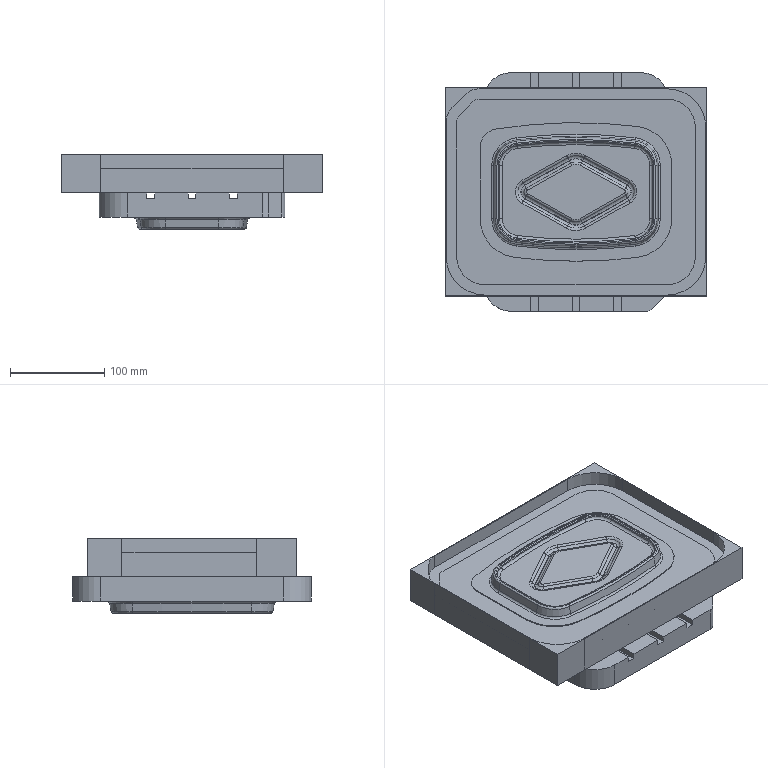NC program | NX | posted with a generic post | part box 278.144 x 254.144 x 79 mm
Lines 4921 to 5862 of 124328:
(CONTOUR_AREA_1 , TOOL : R2)
N9834 M6
N9836 G53
N9838 G17 G0 G90 X-4.674 Y-0.007 S8000 M3 M8
N9840 G43 Z100.5 H0
N9842 Z36.98
N9844 G94 G1 Z33.98 F4500.
N9846 G3 X4.675 Y0.005 R63.773
N9848 G1 X4.673 Y0.006
N9850 G3 X-0.193 Y0.163 R72.733
N9852 X-4.674 Y-0.007 R101.082
N9854 G1 X-8.51 Y-0.148
N9856 X-7.093 Y-0.193
N9858 X-6.747 Y-0.204
N9860 X-5.711 Y-0.244
N9862 G3 X2.733 Y-0.382 R74.506
N9864 G1 X6.059 Y-0.224
N9866 X8.48 Y-0.141
N9868 X11.596 Y-0.07
N9870 X13.848 Y0.003
N9872 X13.852 Y0.004
N9874 X11.743 Y0.077
N9876 G2 X1.804 Y0.42 R263.458
N9878 G3 X-3.288 Y0.349 R55.344
N9880 G1 X-5.646 Y0.238
N9882 X-8.203 Y0.16
N9884 X-13.845 Y0.001
N9886 X-11.249 Y-0.085
N9888 X-8.51 Y-0.148
N9890 X-8.519 Y-0.432
N9892 X-7.056 Y-0.479
N9894 X-6.721 Y-0.49
N9896 X-5.71 Y-0.529
N9898 G3 X2.942 Y-0.657 R74.079
N9900 G1 X5.712 Y-0.522
N9902 X8.576 Y-0.423
N9904 X11.596 Y-0.355
N9906 X20.353 Y-0.069
N9908 X21.805 Y-0.001
N9910 X21.812 Y0.003
N9912 X21.811 Y0.004
N9914 X21.662 Y0.019
N9916 X21.633 Y0.021
N9918 X20.164 Y0.088
N9920 X11.446 Y0.37
N9922 X9.073 Y0.419
N9924 X8.48 Y0.433
N9926 X6.051 Y0.513
N9928 X2.745 Y0.668
N9930 G3 X-2.942 Y0.651 R53.586
N9932 G1 X-5.712 Y0.521
N9934 X-6.784 Y0.485
N9936 X-8.03 Y0.45
N9938 X-16.097 Y0.225
N9940 X-19.624 Y0.105
N9942 X-21.806 Y0.002
N9944 X-20.941 Y-0.044
N9946 X-20.387 Y-0.068
N9948 X-20.153 Y-0.078
N9950 X-11.104 Y-0.373
N9952 X-8.519 Y-0.432
N9954 X-8.528 Y-0.717
N9956 X-7.096 Y-0.763
N9958 X-6.662 Y-0.778
N9960 X-5.711 Y-0.815
N9962 G3 X2.861 Y-0.947 R74.273
N9964 G1 X5.771 Y-0.805
N9966 X8.639 Y-0.707
N9968 X11.596 Y-0.641
N9970 X20.417 Y-0.351
N9972 X22.672 Y-0.244
N9974 X27.347 Y0.002
N9976 X21.101 Y0.333
N9978 X20.105 Y0.375
N9980 X11.387 Y0.656
N9982 X8.134 Y0.728
N9984 X5.993 Y0.801
N9986 X2.596 Y0.96
N9988 X1.015 Y1.014
N9990 X0.331 Y1.023
N9992 X-1.211 Y0.998
N9994 X-2.596 Y0.951
N9996 X-5.773 Y0.804
N9998 X-6.75 Y0.771
N10000 X-8.826 Y0.713
N10002 X-16.104 Y0.51
N10004 X-19.557 Y0.393
N10006 X-22.672 Y0.249
N10008 X-27.341 Y0.006
N10010 X-27.172 Y-0.01
N10012 G3 X-8.528 Y-0.717 R468.382
N10014 G1 X-8.537 Y-1.002
N10016 X-6.057 Y-1.086
N10018 G3 X1.558 Y-1.282 R81.793
N10020 G1 X2.599 Y-1.245
N10022 X5.834 Y-1.088
N10024 X8.345 Y-1.
N10026 G3 X29.624 Y-0.144 R470.604
N10028 G1 X29.619 Y0.027
N10030 X29.594 Y0.147
N10032 X29.578 Y0.157
N10034 X29.416 Y0.173
N10036 X28.21 Y0.244
N10038 G3 X8.134 Y1.014 R451.313
N10040 G1 X5.935 Y1.089
N10042 X4.613 Y1.152
N10044 G3 X-1.905 Y1.263 R62.851
N10046 G1 X-2.253 Y1.251
N10048 X-2.944 Y1.222
N10050 X-5.835 Y1.087
N10052 X-8.826 Y0.997
N10054 G3 X-29.609 Y0.158 R503.183
N10056 G1 X-29.661 Y0.108
N10058 X-29.674 Y0.094
N10060 X-29.655 Y-0.033
N10062 X-29.594 Y-0.142
N10064 X-29.574 Y-0.153
N10066 X-29.364 Y-0.173
N10068 G3 X-8.537 Y-1.002 R491.866
N10070 G1 X-8.546 Y-1.287
N10072 X-6.057 Y-1.372
N10074 G3 X1.214 Y-1.579 R86.109
N10076 G1 X2.624 Y-1.529
N10078 X5.897 Y-1.371
N10080 X8.408 Y-1.283
N10082 G3 X29.683 Y-0.431 R486.038
N10084 G1 X29.842 Y-0.398
N10086 X29.899 Y-0.214
N10088 X29.961 Y0.193
N10090 X29.941 Y0.398
N10092 X29.839 Y0.418
N10094 X29.594 Y0.446
N10096 G3 X8.48 Y1.288 R447.781
N10098 G1 X6.209 Y1.363
N10100 G3 X0.516 Y1.594 R157.649
N10102 X-5.899 Y1.37 R117.358
N10104 G1 X-10.214 Y1.243
N10106 G3 X-29.681 Y0.433 R462.283
N10108 G1 X-29.941 Y0.36
N10110 X-29.973 Y0.141
N10112 X-29.964 Y-0.173
N10114 X-29.963 Y-0.196
N10116 X-29.941 Y-0.335
N10118 X-29.829 Y-0.407
N10120 X-29.594 Y-0.439
N10122 X-29.523 Y-0.447
N10124 G3 X-8.546 Y-1.287 R488.305
N10126 G1 X-8.555 Y-1.571
N10128 X-6.057 Y-1.657
N10130 G3 X1.252 Y-1.863 R85.774
N10132 G1 X2.689 Y-1.811
N10134 X6.057 Y-1.65
N10136 X8.482 Y-1.566
N10138 G3 X30.117 Y-0.689 R483.031
N10140 G1 X30.238 Y0.124
N10142 X30.242 Y0.173
N10144 X30.256 Y0.488
N10146 X30.251 Y0.519
N10148 X30.215 Y0.645
N10150 X30.1 Y0.678
N10152 X29.941 Y0.705
N10154 X29.796 Y0.72
N10156 G3 X19.554 Y1.249 R696.433
N10158 G1 X11.547 Y1.508
N10160 G2 X1.845 Y1.844 R245.456
N10162 G3 X-3.059 Y1.787 R52.345
N10164 G1 X-5.365 Y1.678
N10166 X-5.602 Y1.667
N10168 X-6.057 Y1.65
N10170 X-6.75 Y1.627
N10172 X-16.441 Y1.354
N10174 G3 X-30.117 Y0.689 R351.813
N10176 G1 X-30.153 Y0.668
N10178 X-30.187 Y0.618
N10180 G3 X-30.164 Y-0.626 R2.302
N10182 G1 X-30.097 Y-0.676
N10184 X-29.941 Y-0.699
N10186 X-29.791 Y-0.716
N10188 G3 X-8.555 Y-1.571 R485.815
N10190 G1 X-8.564 Y-1.856
N10192 X-7.431 Y-1.892
N10194 X-6.748 Y-1.915
N10196 X-5.71 Y-1.955
N10198 G3 X2.752 Y-2.093 R74.97
N10200 G1 X5.713 Y-1.948
N10202 X8.534 Y-1.85
N10204 G3 X30.181 Y-0.971 R487.335
N10206 G1 X30.287 Y-0.944
N10208 X30.342 Y-0.923
N10210 X30.363 Y-0.865
N10212 G3 X30.51 Y0.743 R4.48
N10214 G1 X30.483 Y0.865
N10216 X30.46 Y0.937
N10218 X30.381 Y0.959
N10220 X30.287 Y0.972
N10222 X30.066 Y0.991
N10224 G3 X19.199 Y1.546 R638.381
N10226 G1 X11.487 Y1.795
N10228 X8.48 Y1.858
N10230 X6.055 Y1.939
N10232 X2.786 Y2.093
N10234 G3 X-3.288 Y2.061 R55.77
N10236 G1 X-5.714 Y1.946
N10238 X-6.751 Y1.911
N10240 G3 X-27.591 Y1.138 R612.114
N10242 G1 X-29.941 Y0.996
N10244 X-30.175 Y0.977
N10246 X-30.287 Y0.958
N10248 X-30.369 Y0.939
N10250 G3 X-30.535 Y0.173 R1.661
N10252 X-30.415 Y-0.865 R3.329
N10254 G1 X-30.364 Y-0.943
N10256 X-30.287 Y-0.956
N10258 X-30.059 Y-0.984
N10260 G3 X-8.564 Y-1.856 R486.78
N10262 G1 X-8.573 Y-2.141
N10264 X-7.372 Y-2.179
N10266 X-6.702 Y-2.202
N10268 X-5.703 Y-2.241
N10270 G3 X2.454 Y-2.391 R75.415
N10272 G1 X5.711 Y-2.234
N10274 X8.24 Y-2.144
N10276 G3 X30.609 Y-1.235 R485.132
N10278 G1 X30.794 Y-0.012
N10280 G3 X30.71 Y1.211 R2.988
N10282 G1 X30.655 Y1.233
N10284 X30.633 Y1.24
N10286 G3 X8.377 Y2.146 R462.527
N10288 G1 X7.096 Y2.186
N10290 X6.057 Y2.224
N10292 X2.596 Y2.386
N10294 X1.055 Y2.439
N10296 G3 X-5.73 Y2.231 R104.374
N10298 G1 X-6.75 Y2.197
N10300 X-8.024 Y2.16
N10302 G3 X-30.654 Y1.224 R489.99
N10304 G1 X-30.674 Y1.211
N10306 X-30.679 Y1.201
N10308 G3 X-30.654 Y-1.211 R4.623
N10310 G1 X-30.63 Y-1.234
N10312 G3 X-8.573 Y-2.141 R499.854
N10314 G1 X-8.582 Y-2.426
N10316 X-5.977 Y-2.515
N10318 G3 X2.517 Y-2.674 R78.238
N10320 G1 X5.791 Y-2.516
N10322 X8.303 Y-2.427
N10324 G3 X30.681 Y-1.51 R454.807
N10326 G1 X30.839 Y-1.447
N10328 X30.884 Y-1.306
N10330 X31.06 Y-0.173
N10332 G3 X30.979 Y1.472 R4.243
N10334 G1 X30.911 Y1.489
N10336 X30.633 Y1.525
N10338 X30.604 Y1.528
N10340 G3 X8.318 Y2.433 R463.922
N10342 G2 X1.333 Y2.717 R1018.731
N10344 G3 X-5.792 Y2.514 R97.878
N10346 G1 X-9.005 Y2.417
N10348 X-16.124 Y2.22
N10350 G3 X-30.676 Y1.514 R450.176
N10352 G1 X-30.9 Y1.468
N10354 G3 X-31.016 Y-0.902 R4.912
N10356 G1 X-30.969 Y-1.211
N10358 X-30.895 Y-1.473
N10360 X-30.633 Y-1.516
N10362 X-30.596 Y-1.521
N10364 G3 X-8.582 Y-2.426 R535.511
N10366 G1 X-8.591 Y-2.711
N10368 X-6.057 Y-2.797
N10370 G3 X0.093 Y-3.021 R114.841
N10372 G1 X1.147 Y-3.006
N10374 X1.559 Y-2.994
N10376 X2.598 Y-2.957
N10378 X5.854 Y-2.799
N10380 X8.366 Y-2.71
N10382 G3 X31.109 Y-1.773 R498.462
N10384 G1 X31.169 Y-1.368
N10386 X31.354 Y-0.144
N10388 G3 X31.171 Y1.749 R3.772
N10390 G1 X30.979 Y1.779
N10392 X30.868 Y1.793
N10394 G3 X8.595 Y2.711 R488.125
N10396 G1 X6.057 Y2.795
N10398 X2.942 Y2.944
N10400 G3 X-2.95 Y2.933 R60.32
N10402 G1 X-5.855 Y2.797
N10404 X-8.712 Y2.71
N10406 X-16.187 Y2.503
N10408 G3 X-31.12 Y1.763 R360.307
N10410 G1 X-31.148 Y1.737
N10412 X-31.176 Y1.707
N10414 G3 X-31.403 Y0.095 R12.569
N10416 G1 X-31.397 Y-0.173
N10418 G3 X-31.15 Y-1.728 R13.812
N10420 G1 X-30.979 Y-1.764
N10422 X-30.86 Y-1.784
N10424 X-30.633 Y-1.805
N10426 X-30.541 Y-1.811
N10428 G3 X-8.591 Y-2.711 R491.092
N10430 G1 X-8.599 Y-2.995
N10432 X-6.057 Y-3.083
N10434 G3 X2.644 Y-3.24 R79.137
N10436 G1 X5.917 Y-3.081
N10438 X8.482 Y-2.991
N10440 G3 X31.188 Y-2.04 R464.527
N10442 G1 X31.325 Y-2.004
N10444 X31.376 Y-1.903
N10446 X31.378 Y-1.897
N10448 X31.671 Y0.078
N10450 X31.685 Y0.189
N10452 G3 X31.437 Y2.015 R6.557
N10454 G1 X31.325 Y2.034
N10456 X31.135 Y2.059
N10458 X30.165 Y2.128
N10460 G3 X8.48 Y2.998 R457.791
N10462 G1 X6.19 Y3.075
N10464 X2.885 Y3.231
N10466 G3 X-3.014 Y3.216 R52.388
N10468 G1 X-5.919 Y3.08
N10470 X-8.774 Y2.994
N10472 G3 X-30.979 Y2.066 R488.83
N10474 G1 X-31.182 Y2.047
N10476 X-31.325 Y2.014
N10478 X-31.401 Y1.982
N10480 X-31.425 Y1.903
N10482 X-31.458 Y1.77
N10484 G3 X-31.687 Y-0.194 R8.14
N10486 X-31.404 Y-1.982 R20.433
N10488 G1 X-31.325 Y-2.012
N10490 X-31.124 Y-2.048
N10492 X-30.979 Y-2.065
N10494 X-30.808 Y-2.079
N10496 G3 X-8.599 Y-2.995 R496.073
N10498 G1 X-8.608 Y-3.28
N10500 G2 X-2.498 Y-3.535 R232.226
N10502 G3 X2.708 Y-3.522 R54.583
N10504 G1 X6.057 Y-3.361
N10506 X8.492 Y-3.276
N10508 G3 X31.244 Y-2.33 R483.883
N10510 G1 X31.325 Y-2.314
N10512 X31.588 Y-2.249
N10514 X31.665 Y-1.91
N10516 X31.924 Y-0.173
N10518 G3 X31.94 Y0.865 R2.925
N10520 G1 X31.789 Y1.903
N10522 X31.771 Y2.003
N10524 X31.716 Y2.249
N10526 X31.701 Y2.279
N10528 X31.672 Y2.308
N10530 X31.671 Y2.309
N10532 G3 X8.476 Y3.283 R447.69
N10534 G1 X7.093 Y3.327
N10536 X6.132 Y3.362
N10538 X2.827 Y3.518
N10540 G3 X-3.078 Y3.498 R53.09
N10542 G1 X-5.365 Y3.389
N10544 X-5.622 Y3.377
N10546 X-6.057 Y3.36
N10548 X-6.751 Y3.337
N10550 X-16.441 Y3.065
N10552 G3 X-31.671 Y2.295 R357.257
N10554 G1 X-31.937 Y0.519
N10556 G3 X-31.934 Y-0.519 R3.116
N10558 G1 X-31.669 Y-2.301
N10560 G3 X-8.608 Y-3.28 R468.547
N10562 G1 X-8.617 Y-3.565
N10564 X-6.055 Y-3.653
N10566 G3 X2.772 Y-3.804 R78.892
N10568 G1 X5.714 Y-3.66
N10570 X8.554 Y-3.56
N10572 G3 X31.677 Y-2.589 R486.941
N10574 G1 X31.817 Y-2.551
N10576 X31.842 Y-2.512
N10578 X31.882 Y-2.384
N10580 X32.212 Y-0.173
N10582 G3 X32.16 Y1.354 R4.053
N10584 G1 X32.115 Y1.655
N10586 X32.017 Y2.3
N10588 X31.952 Y2.53
N10590 X31.68 Y2.595
N10592 G3 X8.48 Y3.569 R454.797
N10594 G1 X6.055 Y3.65
N10596 X2.768 Y3.806
N10598 G3 X-3.288 Y3.773 R54.485
N10600 G1 X-5.714 Y3.657
N10602 X-6.762 Y3.622
N10604 G3 X-27.61 Y2.85 R613.557
N10606 G1 X-29.817 Y2.719
N10608 X-31.676 Y2.591
N10610 X-31.9 Y2.505
N10612 X-31.953 Y2.313
N10614 X-32.224 Y0.519
N10616 X-32.252 Y0.285
N10618 X-32.257 Y0.173
N10620 X-32.262 Y-0.071
N10622 X-32.221 Y-0.519
N10624 X-31.973 Y-2.205
N10626 X-31.965 Y-2.249
N10628 X-31.91 Y-2.488
N10630 X-31.89 Y-2.544
N10632 X-31.831 Y-2.559
N10634 X-31.671 Y-2.589
N10636 G3 X-11.125 Y-3.509 R483.526
N10638 G1 X-8.617 Y-3.565
N10640 X-8.626 Y-3.85
N10642 X-7.353 Y-3.891
N10644 X-6.683 Y-3.913
N10646 X-5.684 Y-3.953
N10648 G3 X2.835 Y-4.086 R74.992
N10650 G1 X5.747 Y-3.944
N10652 X8.26 Y-3.854
N10654 G3 X32.116 Y-2.843 R485.604
N10656 G1 X32.28 Y-1.641
N10658 X32.5 Y-0.173
N10660 G3 X32.498 Y0.999 R3.723
N10662 G1 X32.313 Y2.249
N10664 X32.271 Y2.503
N10666 X32.252 Y2.595
N10668 X32.204 Y2.782
N10670 X32.017 Y2.837
N10672 G3 X30.284 Y2.978 R15.434
N10674 G1 X28.556 Y3.079
N10676 G3 X8.358 Y3.857 R450.751
N10678 G1 X6.014 Y3.937
N10680 X2.596 Y4.098
N10682 G3 X-3.634 Y4.042 R55.889
N10684 G1 X-5.387 Y3.958
N10686 X-5.75 Y3.941
N10688 X-8.48 Y3.857
N10690 G3 X-32.017 Y2.849 R485.57
N10692 G1 X-32.123 Y2.836
N10694 X-32.151 Y2.81
N10696 X-32.172 Y2.787
N10698 X-32.482 Y0.747
N10700 G3 X-32.449 Y-0.954 R4.562
N10702 G1 X-32.223 Y-2.455
N10704 X-32.195 Y-2.595
N10706 X-32.16 Y-2.738
N10708 X-32.121 Y-2.815
N10710 X-32.017 Y-2.838
N10712 X-31.929 Y-2.853
N10714 X-31.671 Y-2.875
N10716 X-30.632 Y-2.948
N10718 G3 X-11.065 Y-3.796 R553.148
N10720 G1 X-8.626 Y-3.85
N10722 X-8.635 Y-4.135
N10724 X-6.057 Y-4.223
N10726 G3 X2.25 Y-4.396 R81.327
N10728 G1 X2.596 Y-4.384
N10730 X5.81 Y-4.226
N10732 X8.323 Y-4.137
N10734 G3 X32.017 Y-3.134 R482.346
N10736 G1 X32.188 Y-3.117
N10738 X32.364 Y-3.083
N10740 X32.393 Y-2.92
N10742 X32.558 Y-1.709
N10744 X32.788 Y-0.173
N10746 G3 X32.793 Y0.951 R4.063
N10748 G1 X32.549 Y2.595
N10750 X32.523 Y2.755
N10752 X32.486 Y2.941
N10754 X32.459 Y3.037
N10756 X32.43 Y3.085
N10758 X32.364 Y3.101
N10760 X32.202 Y3.126
N10762 G3 X8.299 Y4.144 R467.327
N10764 G1 X5.957 Y4.225
N10766 X4.635 Y4.288
N10768 G3 X-1.904 Y4.4 R63.61
N10770 G1 X-2.25 Y4.389
N10772 X-2.945 Y4.36
N10774 X-5.812 Y4.225
N10776 X-8.313 Y4.147
N10778 X-16.144 Y3.931
N10780 G3 X-32.186 Y3.119 R370.776
N10782 G1 X-32.364 Y3.085
N10784 X-32.421 Y2.941
N10786 X-32.45 Y2.855
N10788 X-32.761 Y0.814
N10790 G3 X-32.788 Y-0.601 R4.217
N10792 G1 X-32.432 Y-3.016
N10794 X-32.364 Y-3.082
N10796 X-32.189 Y-3.113
N10798 X-32.017 Y-3.133
N10800 X-31.876 Y-3.146
N10802 G3 X-8.635 Y-4.135 R474.324
N10804 G1 X-8.64 Y-4.42
N10806 G2 X-2.248 Y-4.687 R258.1
N10808 G3 X5.874 Y-4.509 R77.091
N10810 G1 X8.386 Y-4.42
N10812 G3 X32.625 Y-3.372 R468.01
N10814 G1 X32.778 Y-2.181
N10816 X33.082 Y-0.147
N10818 G3 X33.056 Y1.142 R4.101
N10820 G1 X32.995 Y1.557
N10822 X32.73 Y3.316
N10824 X32.71 Y3.349
N10826 X32.466 Y3.39
N10828 X32.364 Y3.401
N10830 G3 X8.576 Y4.421 R449.932
N10832 G1 X6.057 Y4.506
N10834 G3 X-0.174 Y4.724 R89.122
N10836 X-5.876 Y4.507 R117.911
N10838 G1 X-8.376 Y4.43
N10840 G3 X-32.364 Y3.4 R492.651
N10842 G1 X-32.621 Y3.376
N10844 X-32.639 Y3.36
N10846 X-32.679 Y3.318
N10848 X-32.851 Y2.108
N10850 X-33.096 Y0.479
N10852 G3 X-33.056 Y-0.748 R4.079
N10854 G1 X-32.729 Y-2.967
N10856 X-32.68 Y-3.288
N10858 X-32.654 Y-3.339
N10860 X-32.553 Y-3.367
N10862 X-32.462 Y-3.386
N10864 G3 X-8.913 Y-4.412 R468.429
N10866 G1 X-8.64 Y-4.42
N10868 X-8.648 Y-4.704
N10870 X-6.057 Y-4.794
N10872 G3 X1.211 Y-5.001 R85.892
N10874 G1 X2.663 Y-4.951
N10876 X6.057 Y-4.787
N10878 X8.483 Y-4.702
N10880 G3 X32.71 Y-3.659 R480.537
N10882 G1 X32.856 Y-3.634
N10884 X32.899 Y-3.444
N10886 X33.114 Y-1.845
N10888 X33.365 Y-0.173
N10890 G3 X33.298 Y1.453 R4.448
N10892 G1 X33.023 Y3.288
N10894 X32.971 Y3.549
N10896 X32.947 Y3.634
N10898 X32.738 Y3.661
N10900 G3 X8.478 Y4.709 R454.232
N10902 G1 X6.172 Y4.786
N10904 G3 X-0.182 Y5.009 R89.978
N10906 G1 X-0.534 Y5.003
N10908 X-1.952 Y4.969
N10910 X-3.033 Y4.927
N10912 X-5.939 Y4.79
N10914 X-6.75 Y4.763
N10916 X-8.136 Y4.722
N10918 G3 X-32.713 Y3.662 R495.127
N10920 G1 X-32.902 Y3.634
N10922 X-32.958 Y3.385
N10924 X-33.129 Y2.176
N10926 X-33.375 Y0.546
N10928 G3 X-33.336 Y-0.799 R4.187
N10930 X-32.902 Y-3.634 R29.727
N10932 G1 X-32.732 Y-3.656
N10934 X-32.707 Y-3.659
N10936 G3 X-8.648 Y-4.704 R469.049
N10938 G1 X-8.657 Y-4.989
N10940 X-6.747 Y-5.052
N10942 X-5.783 Y-5.09
N10944 G3 X1.292 Y-5.283 R81.697
N10946 G1 X1.649 Y-5.272
N10948 X2.366 Y-5.248
N10950 X2.727 Y-5.233
N10952 X6.058 Y-5.072
N10954 X8.512 Y-4.986
N10956 G3 X33.125 Y-3.91 R470.839
N10958 G1 X33.136 Y-3.9
N10960 X33.143 Y-3.893
N10962 X33.281 Y-2.716
N10964 X33.453 Y-1.507
N10966 X33.637 Y-0.284
N10968 G3 X33.594 Y1.403 R4.743
N10970 G1 X33.279 Y3.511
N10972 X33.256 Y3.634
N10974 X33.219 Y3.796
N10976 X33.176 Y3.889
N10978 X33.056 Y3.917
N10980 X33.002 Y3.926
N10982 G3 X8.457 Y4.994 R445.719
N10984 G1 X7.093 Y5.037
N10986 X6.057 Y5.075
N10988 X2.809 Y5.231
N10990 G3 X-3.097 Y5.209 R54.529
N10992 G1 X-5.642 Y5.087
N10994 X-8.145 Y5.007
N10996 G3 X-33.056 Y3.92 R485.083
N10998 G1 X-33.126 Y3.91
N11000 X-33.165 Y3.873
N11002 X-33.187 Y3.848
N11004 X-33.407 Y2.244
N11006 X-33.652 Y0.615
N11008 G3 X-33.587 Y-1.051 R5.016
N11010 G1 X-33.319 Y-2.858
N11012 X-33.215 Y-3.634
N11014 X-33.189 Y-3.767
N11016 X-33.161 Y-3.872
N11018 X-33.056 Y-3.905
N11020 X-32.995 Y-3.919
N11022 X-32.71 Y-3.945
N11024 G3 X-8.657 Y-4.989 R469.981
N11026 G1 X-8.666 Y-5.274
N11028 X-7.393 Y-5.315
N11030 X-6.723 Y-5.338
N11032 X-5.709 Y-5.378
N11034 G3 X2.791 Y-5.515 R75.609
N11036 G1 X5.713 Y-5.371
N11038 X8.218 Y-5.28
N11040 G3 X33.192 Y-4.19 R472.035
N11042 G1 X33.402 Y-4.152
N11044 G2 X33.961 Y0.039 R106.628
N11046 G3 X33.908 Y1.211 R4.502
N11048 G1 X33.576 Y3.461
N11050 X33.535 Y3.767
N11052 X33.503 Y3.98
N11054 X33.485 Y4.063
N11056 X33.462 Y4.129
N11058 X33.402 Y4.157
N11060 X33.262 Y4.186
N11062 X33.056 Y4.21
N11064 X32.949 Y4.219
N11066 G3 X8.398 Y5.281 R468.115
N11068 G1 X7.056 Y5.324
N11070 X6.054 Y5.361
N11072 X2.751 Y5.519
N11074 G3 X-3.288 Y5.485 R55.787
N11076 G1 X-5.712 Y5.368
N11078 X-6.782 Y5.332
N11080 X-8.208 Y5.29
N11082 G3 X-33.187 Y4.194 R480.307
N11084 G1 X-33.402 Y4.156
N11086 X-33.453 Y3.98
N11088 X-33.47 Y3.911
N11090 X-33.626 Y2.717
N11092 X-33.931 Y0.683
N11094 G3 X-33.902 Y-0.865 R4.864
N11096 G1 X-33.614 Y-2.807
N11098 X-33.456 Y-4.041
N11100 X-33.402 Y-4.151
N11102 X-33.255 Y-4.178
N11104 X-33.056 Y-4.203
N11106 X-32.944 Y-4.213
N11108 G3 X-8.666 Y-5.274 R470.866
N11110 G1 X-8.675 Y-5.559
N11112 X-5.999 Y-5.651
N11114 G3 X2.854 Y-5.798 R78.386
N11116 G1 X5.767 Y-5.654
N11118 X8.281 Y-5.564
N11120 G3 X33.402 Y-4.466 R480.107
N11122 G1 X33.628 Y-4.446
N11124 X33.641 Y-4.434
N11126 X33.661 Y-4.413
N11128 G2 X34.241 Y-0.026 R97.134
N11130 G3 X34.14 Y1.612 R5.809
N11132 G1 X33.87 Y3.41
N11134 X33.748 Y4.348
N11136 X33.628 Y4.427
N11138 X33.528 Y4.452
N11140 X33.402 Y4.469
N11142 X33.215 Y4.485
N11144 X30.284 Y4.692
N11146 G3 X8.339 Y5.568 R469.691
N11148 G1 X5.996 Y5.649
N11150 X2.596 Y5.81
N11152 G3 X-3.637 Y5.754 R57.256
N11154 G1 X-5.407 Y5.668
N11156 X-5.769 Y5.652
N11158 X-8.271 Y5.573
N11160 G3 X-33.402 Y4.47 R488.172
N11162 G1 X-33.627 Y4.446
N11164 X-33.656 Y4.426
N11166 X-33.705 Y4.369
N11168 G2 X-34.252 Y0.361 R326.895
N11170 G3 X-34.133 Y-1.259 R6.282
N11172 G1 X-33.867 Y-3.06
N11174 X-33.709 Y-4.287
N11176 X-33.695 Y-4.326
N11178 X-33.63 Y-4.421
N11180 X-33.522 Y-4.446
N11182 X-33.402 Y-4.462
N11184 X-33.21 Y-4.48
N11186 G3 X-8.675 Y-5.559 R469.947
N11188 G1 X-8.68 Y-5.844
N11190 X-6.057 Y-5.934
N11192 G3 X2.599 Y-6.096 R81.091
N11194 G1 X5.83 Y-5.937
N11196 X8.344 Y-5.847
N11198 G3 X33.749 Y-4.728 R479.521
N11200 G1 X33.9 Y-4.672
N11202 X33.94 Y-4.479
N11204 G2 X34.523 Y-0.091 R108.433
N11206 G3 X34.436 Y1.557 R5.757
N11208 G1 X34.164 Y3.363
N11210 X34.039 Y4.326
N11212 X33.995 Y4.573
N11214 X33.971 Y4.672
N11216 X33.798 Y4.721
N11218 X33.748 Y4.733
N11220 G3 X8.616 Y5.846 R449.35
N11222 G1 X6.403 Y5.918
N11224 X2.939 Y6.082
N11226 G3 X-2.945 Y6.072 R62.621
N11228 G1 X-5.832 Y5.935
N11230 X-8.334 Y5.857
N11232 G3 X-33.687 Y4.733 R482.21
N11234 G1 X-33.748 Y4.72
N11236 X-33.937 Y4.672
N11238 X-33.986 Y4.434
N11240 G2 X-34.524 Y0.519 R169.986
N11242 G3 X-34.429 Y-1.211 R6.019
N11244 G2 X-33.963 Y-4.541 R271.915
N11246 G1 X-33.935 Y-4.672
N11248 X-33.792 Y-4.716
N11250 X-33.747 Y-4.728
N11252 G3 X-8.68 Y-5.844 R459.252
N11254 G1 X-8.688 Y-6.128
N11256 X-6.057 Y-6.22
N11258 G3 X1.214 Y-6.427 R85.938
N11260 G1 X2.618 Y-6.38
N11262 X5.894 Y-6.22
N11264 X8.407 Y-6.13
N11266 G3 X34.132 Y-4.98 R469.089
N11268 G1 X34.169 Y-4.944
N11270 X34.185 Y-4.927
N11272 G2 X34.806 Y-0.153 R76.219
N11274 G3 X34.773 Y1.211 R4.936
N11276 G1 X34.44 Y3.442
N11278 X34.283 Y4.672
N11280 X34.255 Y4.832
N11282 X34.223 Y4.956
N11284 X34.094 Y4.989
N11286 X34.07 Y4.994
N11288 X30.842 Y5.226
N11290 X28.207 Y5.383
N11292 X20.94 Y5.763
N11294 X17.653 Y5.874
N11296 X11.593 Y6.07
N11298 X8.48 Y6.134
N11300 X6.057 Y6.217
N11302 G3 X-0.176 Y6.435 R87.388
N11304 X-5.896 Y6.218 R116.114
N11306 G1 X-8.134 Y6.147
N11308 G3 X-34.125 Y4.987 R483.173
N11310 G1 X-34.201 Y4.929
N11312 X-34.223 Y4.889
N11314 G2 X-34.818 Y0.487 R124.772
N11316 G1 X-34.841 Y0.117
N11318 X-34.835 Y-0.221
N11320 X-34.787 Y-0.72
N11322 G2 X-34.225 Y-4.803 R147.904
N11324 G1 X-34.198 Y-4.913
N11326 X-34.094 Y-4.973
N11328 X-34.061 Y-4.984
N11330 G3 X-18.864 Y-5.826 R367.563
N11332 G1 X-11.247 Y-6.073
N11334 X-8.887 Y-6.122
N11336 X-8.688 Y-6.128
N11338 X-8.696 Y-6.413
N11340 X-6.057 Y-6.505
N11342 G3 X1.249 Y-6.711 R85.782
N11344 G1 X2.682 Y-6.662
N11346 X6.057 Y-6.498
N11348 X8.482 Y-6.412
N11350 G3 X34.195 Y-5.263 R469.625
N11352 G1 X34.44 Y-5.22
N11354 G2 X35.089 Y-0.173 R71.318
N11356 G3 X35.027 Y1.452 R5.217
N11358 G1 X34.75 Y3.288
N11360 X34.633 Y4.172
N11362 X34.523 Y5.101
N11364 X34.501 Y5.172
N11366 X34.476 Y5.225
N11368 X34.44 Y5.237
N11370 X34.334 Y5.258
N11372 X34.094 Y5.28
N11374 X33.693 Y5.309
N11376 X30.287 Y5.548
N11378 X27.169 Y5.724
N11380 X20.934 Y6.048
N11382 X17.586 Y6.162
N11384 X11.549 Y6.356
N11386 G2 X2.85 Y6.656 R201.264
N11388 G3 X-3.053 Y6.638 R55.104
N11390 G1 X-5.365 Y6.526
N11392 X-5.599 Y6.515
N11394 X-6.057 Y6.497
N11396 X-6.75 Y6.473
N11398 X-16.788 Y6.192
N11400 G3 X-34.189 Y5.269 R415.647
N11402 G1 X-34.44 Y5.227
N11404 X-34.495 Y5.018
N11406 X-34.51 Y4.948
N11408 G2 X-35.1 Y0.519 R78.712
N11410 G3 X-35.021 Y-1.1 R5.588
N11412 G1 X-34.745 Y-2.941
N11414 X-34.631 Y-3.824
N11416 X-34.496 Y-5.08
N11418 X-34.44 Y-5.219
N11420 X-34.32 Y-5.243
N11422 X-34.094 Y-5.272
N11424 X-34.01 Y-5.28
N11426 G3 X-8.696 Y-6.413 R466.877
N11428 G1 X-8.706 Y-6.698
N11430 X-7.433 Y-6.739
N11432 X-6.747 Y-6.762
N11434 X-5.71 Y-6.804
N11436 G3 X2.746 Y-6.944 R76.284
N11438 G1 X5.713 Y-6.797
N11440 X8.532 Y-6.696
N11442 G3 X34.44 Y-5.534 R450.522
N11444 G1 X34.638 Y-5.512
N11446 X34.669 Y-5.491
N11448 X34.707 Y-5.444
N11450 G2 X35.374 Y-0.173 R72.551
N11452 G3 X35.322 Y1.401 R5.473
N11454 G1 X35.007 Y3.508
N11456 X34.889 Y4.428
N11458 X34.787 Y5.388
N11460 X34.716 Y5.494
N11462 X34.687 Y5.506
N11464 X34.601 Y5.525
N11466 G3 X8.437 Y6.705 R446.849
N11468 G1 X7.096 Y6.748
N11470 X6.055 Y6.787
N11472 X2.792 Y6.944
N11474 G3 X-3.117 Y6.92 R56.052
N11476 G1 X-5.713 Y6.794
N11478 X-6.751 Y6.758
N11480 G3 X-27.518 Y5.995 R605.049
N11482 G1 X-29.788 Y5.863
N11484 X-34.44 Y5.539
N11486 X-34.632 Y5.519
N11488 X-34.691 Y5.496
N11490 X-34.752 Y5.398
N11492 G2 X-35.385 Y0.519 R79.648
N11494 G3 X-35.316 Y-1.049 R5.745
N11496 G1 X-35.003 Y-3.158
N11498 X-34.888 Y-4.081
N11500 X-34.751 Y-5.364
N11502 X-34.714 Y-5.486
N11504 X-34.588 Y-5.511
N11506 X-34.44 Y-5.531
N11508 X-34.277 Y-5.546
N11510 G3 X-8.706 Y-6.698 R468.892
N11512 G1 X-8.715 Y-6.983
N11514 X-7.374 Y-7.026
N11516 X-6.705 Y-7.049
N11518 X-5.706 Y-7.089
N11520 G3 X2.809 Y-7.227 R76.217
N11522 G2 X11.781 Y-6.908 R213.308
N11524 G3 X34.702 Y-5.795 R425.053
N11526 G1 X34.787 Y-5.77
N11528 X34.948 Y-5.71
N11530 X34.99 Y-5.507
N11532 G2 X35.641 Y-0.357 R67.895
N11534 G3 X35.634 Y1.211 R5.95
N11536 G2 X35.036 Y5.613 R92.43
N11538 G1 X35.013 Y5.71
N11540 X34.851 Y5.774
N11542 X34.787 Y5.789
N11544 X34.548 Y5.818
N11546 X34.44 Y5.826
N11548 X30.287 Y6.12
N11550 G3 X8.378 Y6.992 R469.068
N11552 G1 X7.096 Y7.033
N11554 X6.057 Y7.072
N11556 X2.733 Y7.231
N11558 G3 X-3.288 Y7.197 R57.165
N11560 G1 X-5.403 Y7.094
N11562 X-5.726 Y7.079
N11564 X-8.229 Y7.
N11566 G3 X-34.694 Y5.802 R482.176
N11568 G1 X-34.787 Y5.777
N11570 X-34.985 Y5.71
N11572 X-35.033 Y5.463
N11574 G2 X-35.654 Y0.689 R69.659
N11576 G3 X-35.611 Y-0.998 R6.028
N11578 G2 X-35.041 Y-5.364 R58.574
N11580 G1 X-35.008 Y-5.586
N11582 X-34.981 Y-5.71
N11584 X-34.845 Y-5.769
N11586 X-34.787 Y-5.783
N11588 X-34.543 Y-5.812
N11590 G3 X-20.14 Y-6.639 R374.46
N11592 G1 X-11.424 Y-6.923
N11594 X-8.715 Y-6.983
N11596 X-8.72 Y-7.268
N11598 X-5.981 Y-7.363
N11600 G3 X2.942 Y-7.506 R78.663
N11602 G1 X5.787 Y-7.365
N11604 X8.301 Y-7.273
N11606 G3 X35.149 Y-6.056 R481.317
N11608 G1 X35.211 Y-5.987
N11610 X35.233 Y-5.956
N11612 G2 X35.908 Y-0.519 R69.636
N11614 G3 X35.825 Y1.91 R7.249
N11616 G1 X35.553 Y3.713
N11618 X35.434 Y4.672
N11620 X35.326 Y5.71
N11622 X35.299 Y5.877
N11624 X35.277 Y5.955
N11626 X35.186 Y6.056
N11628 X30.94 Y6.363
N11630 G3 X20.091 Y6.936 R542.86
N11632 G1 X11.708 Y7.207
N11634 X8.48 Y7.275
N11636 X6.311 Y7.347
N11638 G3 X-0.388 Y7.571 R90.93
N11640 G1 X-1.904 Y7.538
N11642 X-2.942 Y7.499
N11644 X-5.789 Y7.362
N11646 X-8.134 Y7.288
N11648 G3 X-35.229 Y6.056 R492.943
N11650 G1 X-35.269 Y5.92
N11652 G2 X-35.935 Y0.755 R70.137
N11654 G3 X-35.907 Y-0.95 R6.504
N11656 G1 X-35.55 Y-3.359
N11658 X-35.433 Y-4.326
N11660 X-35.279 Y-5.857
N11662 X-35.258 Y-5.948
N11664 X-35.245 Y-5.982
N11666 X-35.141 Y-6.056
N11668 G3 X-8.72 Y-7.268 R470.637
N11670 G1 X-8.728 Y-7.553
N11672 G2 X-2.247 Y-7.824 R265.776
N11674 G1 X-1.557 Y-7.846
N11676 X0.173 Y-7.867
N11678 X1.558 Y-7.842
N11680 X2.599 Y-7.808
N11682 X5.85 Y-7.647
N11684 X8.364 Y-7.556
N11686 G3 X35.199 Y-6.335 R476.305
N11688 G1 X35.479 Y-6.289
N11690 X35.516 Y-6.056
N11692 G2 X36.202 Y-0.488 R65.683
N11694 G3 X36.171 Y1.518 R6.736
N11696 G1 X35.848 Y3.663
N11698 X35.732 Y4.579
N11700 X35.569 Y6.146
N11702 X35.547 Y6.225
N11704 X35.52 Y6.293
N11706 X35.479 Y6.307
N11708 X35.4 Y6.324
N11710 G3 X19.557 Y7.239 R383.391